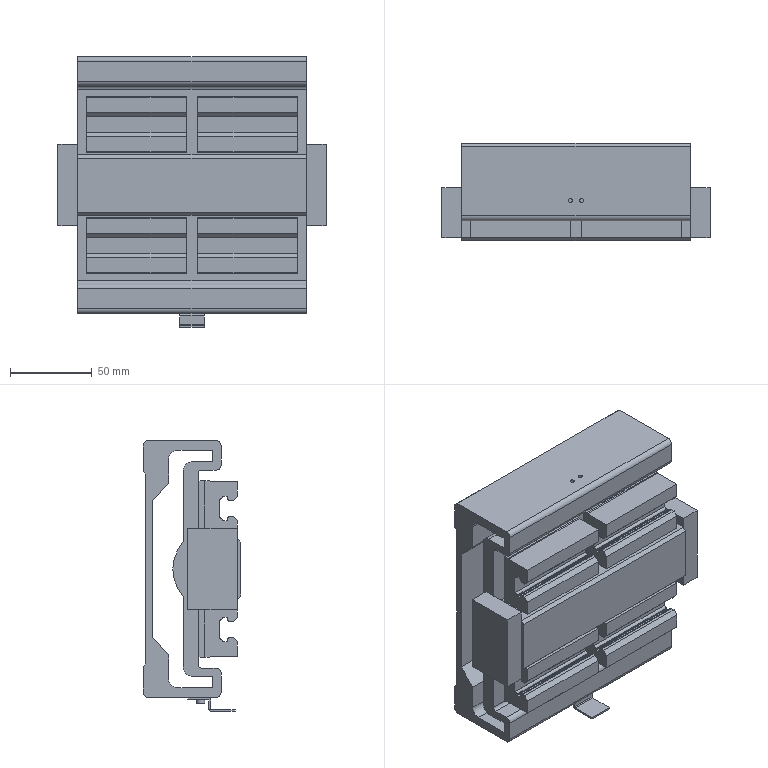Part | NX | features BREP 10 | 10 solids | 489 faces | box 164 x 59.5 x 165.5 mm | volume 699391 mm3 | plane 289 | cylinder 140 | cone 56 | torus 4 | commonest cylinder face diameters 0.4 x32 3.3 x32 5 x24 3 x23 2.5 x8 3.2 x6